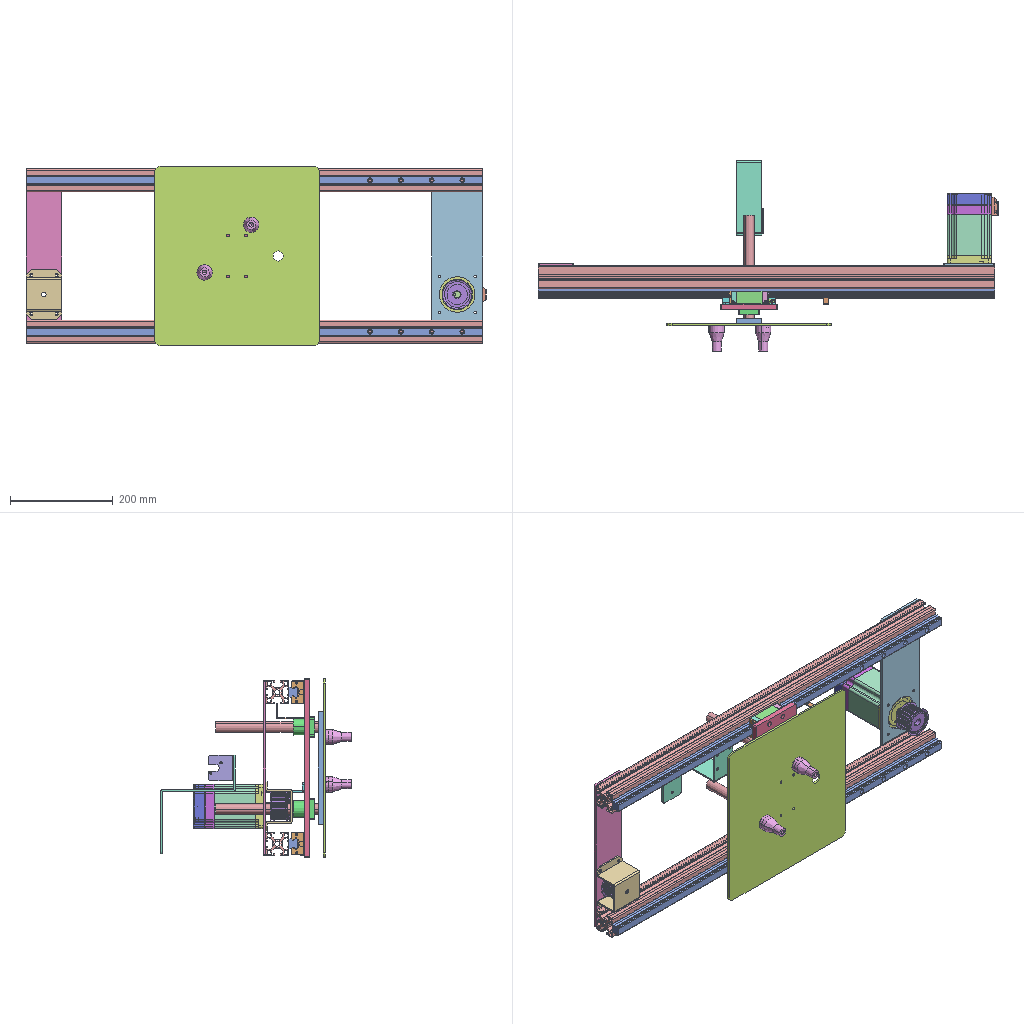Assembly | SolidWorks | 20 different items | 27 placed | box 896 x 371 x 350 mm
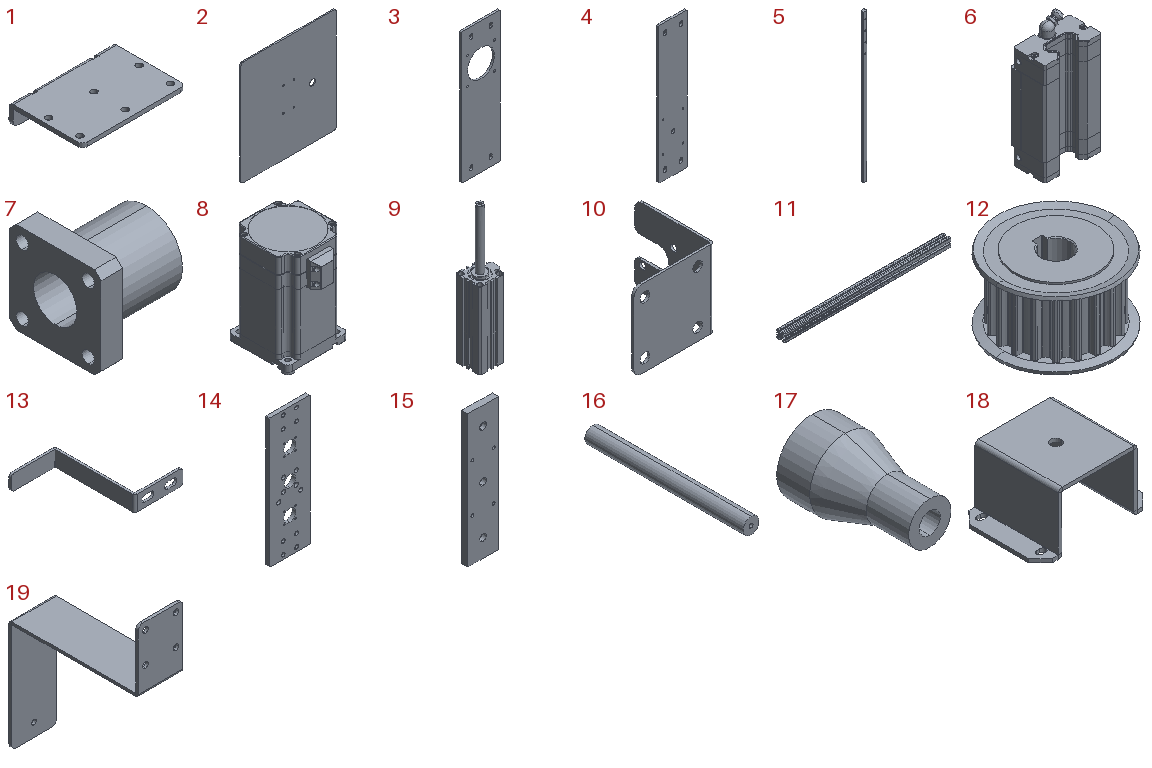Parts list (item | name | quantity | size | volume | features):
1 | - | x1 | 103 x 73 x 20 mm | 35104 mm3 | features ICE 3, EdgeFlange 1, Fillet 1, FlatPattern 1, SMBaseFlange 1, SheetMetal 1
2 | - | x1 | 320 x 4 x 350 mm | 446060 mm3 | features Extrusion 1, Fillet 1, HoleWzd 1, ICE 1
3 | - | x1 | 100 x 5 x 340 mm | 148613 mm3 | features HoleWzd 2, Chamfer 1, Extrusion 1, ICE 1
4 | - | x1 | 70 x 5 x 340 mm | 116578 mm3 | features HoleWzd 2, Chamfer 1, Extrusion 1, ICE 1
5 | - | x2 | 20 x 17.5 x 890 mm | 276758 mm3 | features ICE 15, Chamfer 3, Extrusion 3, Fillet 3, MirrorPattern 3, MirrorSolid 3, RevCut 3, LPattern 2, DeleteBody 1, Dome 1
6 | - | x2 | 44 x 25.7 x 88.7 mm | 65250 mm3 | features ICE 23, Extrusion 5, MirrorPattern 5, Fillet 4, MirrorSolid 4, Chamfer 3, Dome 2, Revolution 2, LibraryFeature 1, RevCut 1
7 | - | x2 | 42 x 42 x 42 mm | 30685 mm3 | features ICE 2, Chamfer 1, Extrusion 1, HoleWzd 1
8 | - | x1 | 85.85 x 99 x 176 mm | 601828 mm3 | features BaseBody 6
9 | - | x1 | 50 x 44 x 241.5 mm | 235412 mm3 | features BaseBody 2, MoveCopyBody 1
10 | - | x1 | 52 x 50 x 50 mm | 6790 mm3 | features Fillet 2, HoleWzd 2, ICE 2, EdgeFlange 1, FlatPattern 1, SMBaseFlange 1, SheetMetal 1
11 | - | x2 | 890 x 45 x 45 mm | 616138 mm3 | features WeldMemberFeat 1, WeldmentFeature 1
12 | - | x2 | 58 x 58 x 33.085 mm | 51729 mm3 | features MBimport 1
13 | - | x1 | 60 x 53.5 x 10 mm | 1574 mm3 | features BreakCorner 1, FlatPattern 1, HoleWzd 1, SMBaseFlange 1, SheetMetal 1
14 | - | x1 | 110 x 10 x 350 mm | 350704 mm3 | features HoleWzd 4, ICE 2, Chamfer 1, Extrusion 1
15 | - | x1 | 50 x 10 x 220 mm | 106947 mm3 | features HoleWzd 2, Extrusion 1
16 | - | x2 | 20 x 200 x 20 mm | 62527 mm3 | features Extrusion 1, HoleWzd 1
17 | - | x2 | 30 x 50 x 30 mm | 17999 mm3 | features HoleWzd 2, Revolution 1
18 | - | x1 | 96 x 70 x 51 mm | 38537 mm3 | features EdgeFlange 3, ICE 2, Chamfer 1, FlatPattern 1, SMBaseFlange 1, SheetMetal 1
19 | - | x1 | 50 x 145 x 192 mm | 49401 mm3 | features EdgeFlange 2, HoleWzd 2, Fillet 1, FlatPattern 1, SMBaseFlange 1, SheetMetal 1
20 | MTHA-1-D6-S6_base | x1 | - | - | -
Mates (type | each side: item.copy, entity, surface, feature):
Coincident | 5.1 face plane Boss-Extrude8 | 6.1 face plane Cut-Extrude11 | 2 times
Coincident | 5.2 face plane Boss-Extrude8 | 5.1 face plane Boss-Extrude8
Coincident | 5.2 face plane Boss-Extrude8 | 6.2 face plane Cut-Extrude11 | 2 times
Coincident | 6.1 face plane Boss-Extrude5 | 6.2 face plane Boss-Extrude5
Coincident | 6.1 face plane Boss-Extrude1 | 14.1 face plane Boss-Extrude1
Concentric | 6.1 face cylinder Mirror2 | 14.1 face cylinder Hole Size (% by) Socket Head Cap Screw Type1 | 2 times
Coincident | 5.2 face plane Boss-Extrude8 | 3.1 face plane Boss-Extrude1
Concentric | 3.1 face cylinder Cut-Extrude1 | 8.1 face cylinder
Parallel | 3.1 face plane Boss-Extrude1 | 8.1 face plane
Concentric | 4.1 face cylinder Cut-Extrude1 | 18.1 face cylinder Cut-Extrude1
Parallel | 4.1 face plane Boss-Extrude1 | 18.1 face plane Edge-Flange1
Coincident | 14.1 face plane Boss-Extrude1 | 1.1 face plane Edge-Flange1
Concentric | 8.1 face cylinder | 12.1 face cylinder EBL33-S8M250-20-A-N-d14.stp
Concentric | 18.1 face cylinder Cut-Extrude1 | 12.2 face cylinder EBL33-S8M250-20-A-N-d14.stp
Concentric | 14.1 face cylinder Cut-Extrude1 | 7.1 face cylinder Cut-Extrude1
Concentric | 14.1 face cylinder Cut-Extrude1 | 7.2 face cylinder Cut-Extrude1
Concentric | 14.1 face cylinder M5 Tapped Hole1 | 7.1 face cylinder Ø5.5 (5.5) Diameter Hole1
Concentric | 14.1 face cylinder M5 Tapped Hole1 | 7.2 face cylinder Ø5.5 (5.5) Diameter Hole1
Concentric | 7.1 face cylinder Cut-Extrude1 | 16.1 face cylinder Boss-Extrude1
Concentric | 7.2 face cylinder Cut-Extrude1 | 16.2 face cylinder Boss-Extrude1
Coincident | 16.1 face plane Boss-Extrude1 | 16.2 face plane Boss-Extrude1
Coincident | 16.2 face plane Boss-Extrude1 | 15.1 face plane Boss-Extrude1
Concentric | 16.2 face cylinder Boss-Extrude1 | 15.1 face cylinder Hole Size (% by) Socket Head Cap Screw Type1
Concentric | 16.1 face cylinder Boss-Extrude1 | 15.1 face cylinder Hole Size (% by) Socket Head Cap Screw Type1
Coincident | 4.1 face plane Boss-Extrude1 | 18.1 face plane Edge-Flange3
Coincident | 11.1 face plane Aluminum Profile 45 X 45L X R2.5(1) | 3.1 face plane Boss-Extrude1 | 3 times
DistanceDim | 5.2 face plane Boss-Extrude8 | 11.1 face plane Aluminum Profile 45 X 45L X R2.5(1)
Coincident | 11.1 face plane Aluminum Profile 45 X 45L X R2.5(1) | 5.2 face plane Boss-Extrude8
DistanceDim | 11.2 face plane Aluminum Profile 45 X 45L X R2.5(1) | 5.1 face plane Boss-Extrude8
Coincident | 11.2 face plane Aluminum Profile 45 X 45L X R2.5(1) | 3.1 face plane Boss-Extrude1 | 2 times
Coincident | 11.1 face plane Aluminum Profile 45 X 45L X R2.5(1) | 11.2 face plane Aluminum Profile 45 X 45L X R2.5(1)
Coincident | 11.2 face plane Aluminum Profile 45 X 45L X R2.5(1) | 5.1 face plane Boss-Extrude8
Coincident | 3.1 face plane Boss-Extrude1 | 8.1 face plane
Coincident | 15.1 face plane Boss-Extrude1 | 2.1 face plane Boss-Extrude1
Concentric | 15.1 face cylinder M6 Tapped Hole1 | 2.1 face cylinder Ø5.2 (5.2) Diameter Hole1 | 2 times
Coincident | 2.1 face plane Boss-Extrude1 | 17.1 face plane Revolve1
Coincident | 2.1 face plane Boss-Extrude1 | 17.2 face plane Revolve1
Coincident | 11.1 face plane Aluminum Profile 45 X 45L X R2.5(1) | 4.1 face plane Boss-Extrude1 | 3 times
Concentric | 14.1 face cylinder Hole Size (% by) Socket Head Cap Screw Type3 | 1.1 face cylinder Cut-Extrude1 | 2 times
Coincident | 14.1 face plane Boss-Extrude1 | 9.1 face plane SDA Ultra-Thin Cylinder Series [SDAS 32×100]_SDA20-100 Ultra-Thin Cylinder-Cylinder-1-solid1
Concentric | 14.1 face cylinder Cut-Extrude2 | 9.1 face cylinder SDA Ultra-Thin Cylinder Series [SDAS 32×100]_SDA20-100 Ultra-Thin Cylinder-Rod-1-solid1
Concentric | 14.1 face cylinder Hole Size (% by) Socket Head Cap Screw Type2 | 9.1 face cylinder SDA Ultra-Thin Cylinder Series [SDAS 32×100]_SDA20-100 Ultra-Thin Cylinder-Cylinder-1-solid1
Coincident | 14.1 face plane Boss-Extrude1 | 7.2 face plane Boss-Extrude1
Coincident | 14.1 face plane Boss-Extrude1 | 7.1 face plane Boss-Extrude1
DistanceDim | 15.1 face plane Boss-Extrude1 | 9.1 face plane SDA Ultra-Thin Cylinder Series [SDAS 32×100]_SDA20-100 Ultra-Thin Cylinder-Rod-1-solid1
Coincident | 9.1 face plane SDA Ultra-Thin Cylinder Series [SDAS 32×100]_SDA20-100 Ultra-Thin Cylinder-Cylinder-1-solid1 | 19.1 face plane Base-Flange1
Concentric | 9.1 face cylinder SDA Ultra-Thin Cylinder Series [SDAS 32×100]_SDA20-100 Ultra-Thin Cylinder-Cylinder-1-solid1 | 19.1 face cylinder Ø6.2 (6.2) Diameter Hole1 | 2 times
Coincident | 14.1 face plane Boss-Extrude1 | 13.1 face plane Base-Flange1
Coincident | 19.1 face plane Base-Flange1 | 10.1 face plane Base-Flange1
Concentric | 19.1 face cylinder Ø6.2 (6.2) Diameter Hole1 | 10.1 face cylinder Ø6.2 (6.2) Diameter Hole1 | 2 times